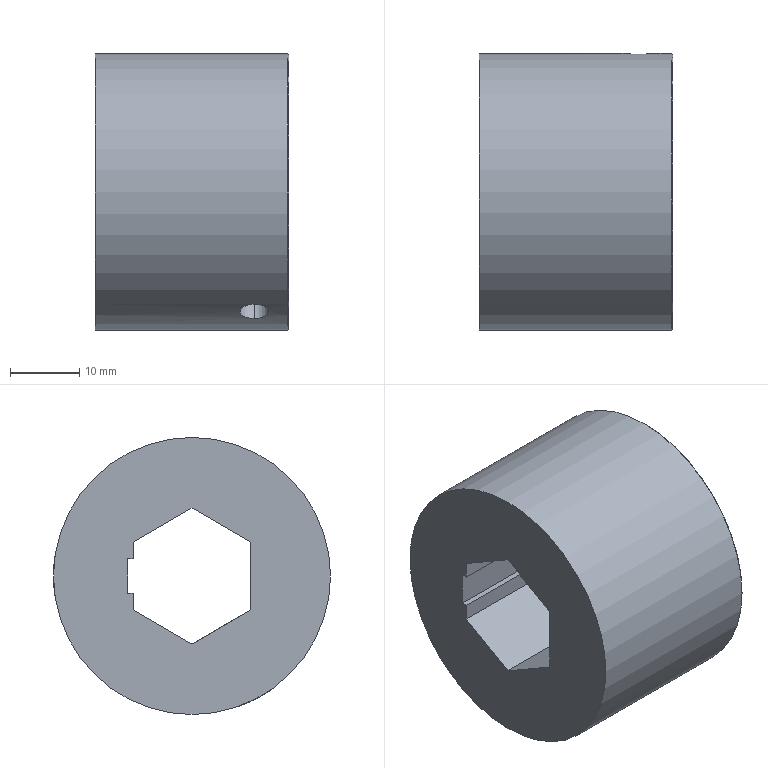Part | STEP file | ATP40XL050-B-hex socket | 1 solid | 19 faces | box 28 x 40 x 40 mm | volume 27766 mm3 | plane 12 | cylinder 5 | cone 2 | commonest cylinder face diameters 4.134 x4 40 x1
STEP:
#1=CARTESIAN_POINT('',(0.,8.5,-2.5));
#2=VERTEX_POINT('',#1);
#3=CARTESIAN_POINT('',(0.,8.5,-4.907));
#4=VERTEX_POINT('',#3);
#5=CARTESIAN_POINT('',(0.,8.5,0.));
#6=DIRECTION('',(0.,0.,-1.));
#7=VECTOR('',#6,1000.);
#8=LINE('',#5,#7);
#9=EDGE_CURVE('',#2,#4,#8,.T.);
#10=ORIENTED_EDGE('',*,*,#9,.F.);
#11=CARTESIAN_POINT('',(0.,9.3,-2.5));
#12=VERTEX_POINT('',#11);
#13=CARTESIAN_POINT('',(0.,13.65,-2.5));
#14=DIRECTION('',(0.,1.,0.));
#15=VECTOR('',#14,1000.);
#16=LINE('',#13,#15);
#17=EDGE_CURVE('',#2,#12,#16,.T.);
#18=ORIENTED_EDGE('',*,*,#17,.T.);
#19=CARTESIAN_POINT('',(0.,9.3,2.5));
#20=VERTEX_POINT('',#19);
#21=CARTESIAN_POINT('',(0.,9.3,1.25));
#22=DIRECTION('',(0.,0.,1.));
#23=VECTOR('',#22,1000.);
#24=LINE('',#21,#23);
#25=EDGE_CURVE('',#12,#20,#24,.T.);
#26=ORIENTED_EDGE('',*,*,#25,.T.);
#27=CARTESIAN_POINT('',(0.,8.5,2.5));
#28=VERTEX_POINT('',#27);
#29=CARTESIAN_POINT('',(0.,9.,2.5));
#30=DIRECTION('',(0.,-1.,0.));
#31=VECTOR('',#30,1000.);
#32=LINE('',#29,#31);
#33=EDGE_CURVE('',#20,#28,#32,.T.);
#34=ORIENTED_EDGE('',*,*,#33,.T.);
#35=CARTESIAN_POINT('',(0.,8.5,4.907));
#36=VERTEX_POINT('',#35);
#37=CARTESIAN_POINT('',(0.,8.5,4.907));
#38=DIRECTION('',(0.,0.,-1.));
#39=VECTOR('',#38,1000.);
#40=LINE('',#37,#39);
#41=EDGE_CURVE('',#36,#28,#40,.T.);
#42=ORIENTED_EDGE('',*,*,#41,.F.);
#43=CARTESIAN_POINT('',(0.,0.,9.815));
#44=VERTEX_POINT('',#43);
#45=CARTESIAN_POINT('',(0.,0.,9.815));
#46=DIRECTION('',(0.,0.866,-0.5));
#47=VECTOR('',#46,1000.);
#48=LINE('',#45,#47);
#49=EDGE_CURVE('',#44,#36,#48,.T.);
#50=ORIENTED_EDGE('',*,*,#49,.F.);
#51=CARTESIAN_POINT('',(0.,-8.5,4.907));
#52=VERTEX_POINT('',#51);
#53=CARTESIAN_POINT('',(0.,-8.5,4.907));
#54=DIRECTION('',(0.,0.866,0.5));
#55=VECTOR('',#54,1000.);
#56=LINE('',#53,#55);
#57=EDGE_CURVE('',#52,#44,#56,.T.);
#58=ORIENTED_EDGE('',*,*,#57,.F.);
#59=CARTESIAN_POINT('',(0.,-8.5,-4.907));
#60=VERTEX_POINT('',#59);
#61=CARTESIAN_POINT('',(0.,-8.5,-4.907));
#62=DIRECTION('',(0.,0.,1.));
#63=VECTOR('',#62,1000.);
#64=LINE('',#61,#63);
#65=EDGE_CURVE('',#60,#52,#64,.T.);
#66=ORIENTED_EDGE('',*,*,#65,.F.);
#67=CARTESIAN_POINT('',(0.,0.,-9.815));
#68=VERTEX_POINT('',#67);
#69=CARTESIAN_POINT('',(0.,0.,-9.815));
#70=DIRECTION('',(0.,-0.866,0.5));
#71=VECTOR('',#70,1000.);
#72=LINE('',#69,#71);
#73=EDGE_CURVE('',#68,#60,#72,.T.);
#74=ORIENTED_EDGE('',*,*,#73,.F.);
#75=CARTESIAN_POINT('',(0.,8.5,-4.907));
#76=DIRECTION('',(0.,-0.866,-0.5));
#77=VECTOR('',#76,1000.);
#78=LINE('',#75,#77);
#79=EDGE_CURVE('',#4,#68,#78,.T.);
#80=ORIENTED_EDGE('',*,*,#79,.F.);
#81=EDGE_LOOP('',(#10,#18,#26,#34,#42,#50,#58,#66,#74,#80));
#82=FACE_BOUND('',#81,.T.);
#83=CARTESIAN_POINT('',(0.,0.,-20.));
#84=VERTEX_POINT('',#83);
#85=CARTESIAN_POINT('',(0.,0.,0.));
#86=DIRECTION('',(1.,0.,0.));
#87=DIRECTION('',(0.,0.,-1.));
#88=AXIS2_PLACEMENT_3D('',#85,#86,#87);
#89=CIRCLE('',#88,20.);
#90=EDGE_CURVE('',#84,#84,#89,.T.);
#91=ORIENTED_EDGE('',*,*,#90,.F.);
#92=EDGE_LOOP('',(#91));
#93=FACE_OUTER_BOUND('',#92,.T.);
#94=CARTESIAN_POINT('',(0.,18.,0.));
#95=DIRECTION('',(-1.,0.,0.));
#96=DIRECTION('',(0.,0.,1.));
#97=AXIS2_PLACEMENT_3D('',#94,#95,#96);
#98=PLANE('',#97);
#99=ADVANCED_FACE('',(#82,#93),#98,.T.);
#100=CARTESIAN_POINT('',(28.,19.8,0.));
#101=VERTEX_POINT('',#100);
#102=CARTESIAN_POINT('',(27.8,20.,0.));
#103=VERTEX_POINT('',#102);
#104=CARTESIAN_POINT('',(27.9,19.9,0.));
#105=DIRECTION('',(-0.7071,0.7071,0.));
#106=VECTOR('',#105,1000.);
#107=LINE('',#104,#106);
#108=EDGE_CURVE('',#101,#103,#107,.T.);
#109=ORIENTED_EDGE('',*,*,#108,.F.);
#110=CARTESIAN_POINT('',(28.,-19.8,0.));
#111=VERTEX_POINT('',#110);
#112=CARTESIAN_POINT('',(28.,0.,0.));
#113=DIRECTION('',(-1.,0.,0.));
#114=DIRECTION('',(0.,1.,0.));
#115=AXIS2_PLACEMENT_3D('',#112,#113,#114);
#116=CIRCLE('',#115,19.8);
#117=EDGE_CURVE('',#101,#111,#116,.T.);
#118=ORIENTED_EDGE('',*,*,#117,.T.);
#119=CARTESIAN_POINT('',(27.8,-20.,0.));
#120=VERTEX_POINT('',#119);
#121=CARTESIAN_POINT('',(27.9,-19.9,0.));
#122=DIRECTION('',(0.7071,0.7071,0.));
#123=VECTOR('',#122,1000.);
#124=LINE('',#121,#123);
#125=EDGE_CURVE('',#120,#111,#124,.T.);
#126=ORIENTED_EDGE('',*,*,#125,.F.);
#127=CARTESIAN_POINT('',(27.8,0.,0.));
#128=DIRECTION('',(-1.,0.,0.));
#129=DIRECTION('',(0.,1.,0.));
#130=AXIS2_PLACEMENT_3D('',#127,#128,#129);
#131=CIRCLE('',#130,20.);
#132=EDGE_CURVE('',#103,#120,#131,.T.);
#133=ORIENTED_EDGE('',*,*,#132,.F.);
#134=EDGE_LOOP('',(#109,#118,#126,#133));
#135=FACE_OUTER_BOUND('',#134,.T.);
#136=CARTESIAN_POINT('',(27.9,0.,0.));
#137=DIRECTION('',(-1.,0.,0.));
#138=DIRECTION('',(0.,1.,0.));
#139=AXIS2_PLACEMENT_3D('',#136,#137,#138);
#140=CONICAL_SURFACE('',#139,19.9,0.7854);
#141=ADVANCED_FACE('',(#135),#140,.T.);
#142=CARTESIAN_POINT('',(23.,19.893,-2.067));
#143=VERTEX_POINT('',#142);
#144=CARTESIAN_POINT('',(25.067,20.,0.));
#145=VERTEX_POINT('',#144);
#146=CARTESIAN_POINT('',(23.,19.893,-2.067));
#147=CARTESIAN_POINT('',(23.274,19.893,-2.067));
#148=CARTESIAN_POINT('',(23.538,19.899,-2.014));
#149=CARTESIAN_POINT('',(24.044,19.919,-1.805));
#150=CARTESIAN_POINT('',(24.268,19.932,-1.655));
#151=CARTESIAN_POINT('',(24.655,19.961,-1.268));
#152=CARTESIAN_POINT('',(24.805,19.974,-1.045));
#153=CARTESIAN_POINT('',(25.015,19.994,-0.538));
#154=CARTESIAN_POINT('',(25.067,20.,-0.2742));
#155=CARTESIAN_POINT('',(25.067,20.,0.));
#156=B_SPLINE_CURVE_WITH_KNOTS('',3,(#146,#147,#148,#149,#150,#151,#152,#153,#154,#155),.UNSPECIFIED.,.F.,.F.,(4,2,2,2,4),(0.,0.25,0.5,0.75,1.),.UNSPECIFIED.);
#157=EDGE_CURVE('',#143,#145,#156,.T.);
#158=ORIENTED_EDGE('',*,*,#157,.T.);
#159=CARTESIAN_POINT('',(23.,19.893,2.067));
#160=VERTEX_POINT('',#159);
#161=CARTESIAN_POINT('',(25.067,20.,0.));
#162=CARTESIAN_POINT('',(25.067,20.,0.2741));
#163=CARTESIAN_POINT('',(25.014,19.994,0.5381));
#164=CARTESIAN_POINT('',(24.805,19.974,1.044));
#165=CARTESIAN_POINT('',(24.655,19.961,1.268));
#166=CARTESIAN_POINT('',(24.268,19.932,1.655));
#167=CARTESIAN_POINT('',(24.044,19.919,1.805));
#168=CARTESIAN_POINT('',(23.538,19.899,2.014));
#169=CARTESIAN_POINT('',(23.274,19.893,2.067));
#170=CARTESIAN_POINT('',(23.,19.893,2.067));
#171=B_SPLINE_CURVE_WITH_KNOTS('',3,(#161,#162,#163,#164,#165,#166,#167,#168,#169,#170),.UNSPECIFIED.,.F.,.F.,(4,2,2,2,4),(0.,0.25,0.5,0.75,1.),.UNSPECIFIED.);
#172=EDGE_CURVE('',#145,#160,#171,.T.);
#173=ORIENTED_EDGE('',*,*,#172,.T.);
#174=CARTESIAN_POINT('',(20.933,20.,0.));
#175=VERTEX_POINT('',#174);
#176=CARTESIAN_POINT('',(23.,19.893,2.067));
#177=CARTESIAN_POINT('',(22.726,19.893,2.067));
#178=CARTESIAN_POINT('',(22.462,19.899,2.014));
#179=CARTESIAN_POINT('',(21.956,19.919,1.805));
#180=CARTESIAN_POINT('',(21.732,19.932,1.655));
#181=CARTESIAN_POINT('',(21.345,19.961,1.268));
#182=CARTESIAN_POINT('',(21.195,19.974,1.045));
#183=CARTESIAN_POINT('',(20.985,19.994,0.538));
#184=CARTESIAN_POINT('',(20.933,20.,0.2742));
#185=CARTESIAN_POINT('',(20.933,20.,0.));
#186=B_SPLINE_CURVE_WITH_KNOTS('',3,(#176,#177,#178,#179,#180,#181,#182,#183,#184,#185),.UNSPECIFIED.,.F.,.F.,(4,2,2,2,4),(0.,0.25,0.5,0.75,1.),.UNSPECIFIED.);
#187=EDGE_CURVE('',#160,#175,#186,.T.);
#188=ORIENTED_EDGE('',*,*,#187,.T.);
#189=CARTESIAN_POINT('',(20.933,20.,0.));
#190=CARTESIAN_POINT('',(20.933,20.,-0.2741));
#191=CARTESIAN_POINT('',(20.986,19.994,-0.5381));
#192=CARTESIAN_POINT('',(21.195,19.974,-1.044));
#193=CARTESIAN_POINT('',(21.345,19.961,-1.268));
#194=CARTESIAN_POINT('',(21.732,19.932,-1.655));
#195=CARTESIAN_POINT('',(21.956,19.919,-1.805));
#196=CARTESIAN_POINT('',(22.462,19.899,-2.014));
#197=CARTESIAN_POINT('',(22.726,19.893,-2.067));
#198=CARTESIAN_POINT('',(23.,19.893,-2.067));
#199=B_SPLINE_CURVE_WITH_KNOTS('',3,(#189,#190,#191,#192,#193,#194,#195,#196,#197,#198),.UNSPECIFIED.,.F.,.F.,(4,2,2,2,4),(0.,0.25,0.5,0.75,1.),.UNSPECIFIED.);
#200=EDGE_CURVE('',#175,#143,#199,.T.);
#201=ORIENTED_EDGE('',*,*,#200,.T.);
#202=EDGE_LOOP('',(#158,#173,#188,#201));
#203=FACE_BOUND('',#202,.T.);
#204=ORIENTED_EDGE('',*,*,#132,.T.);
#205=CARTESIAN_POINT('',(27.8,0.,0.));
#206=DIRECTION('',(-1.,0.,0.));
#207=DIRECTION('',(0.,1.,0.));
#208=AXIS2_PLACEMENT_3D('',#205,#206,#207);
#209=CIRCLE('',#208,20.);
#210=EDGE_CURVE('',#120,#103,#209,.T.);
#211=ORIENTED_EDGE('',*,*,#210,.T.);
#212=EDGE_LOOP('',(#204,#211));
#213=FACE_OUTER_BOUND('',#212,.T.);
#214=CARTESIAN_POINT('',(25.067,-10.,-17.321));
#215=VERTEX_POINT('',#214);
#216=CARTESIAN_POINT('',(23.,-8.156,-18.261));
#217=VERTEX_POINT('',#216);
#218=CARTESIAN_POINT('',(25.067,-10.,-17.321));
#219=CARTESIAN_POINT('',(25.067,-9.763,-17.458));
#220=CARTESIAN_POINT('',(25.014,-9.531,-17.585));
#221=CARTESIAN_POINT('',(24.805,-9.083,-17.82));
#222=CARTESIAN_POINT('',(24.655,-8.882,-17.92));
#223=CARTESIAN_POINT('',(24.268,-8.533,-18.09));
#224=CARTESIAN_POINT('',(24.044,-8.397,-18.152));
#225=CARTESIAN_POINT('',(23.538,-8.205,-18.24));
#226=CARTESIAN_POINT('',(23.274,-8.156,-18.261));
#227=CARTESIAN_POINT('',(23.,-8.156,-18.261));
#228=B_SPLINE_CURVE_WITH_KNOTS('',3,(#218,#219,#220,#221,#222,#223,#224,#225,#226,#227),.UNSPECIFIED.,.F.,.F.,(4,2,2,2,4),(0.,0.25,0.5,0.75,1.),.UNSPECIFIED.);
#229=EDGE_CURVE('',#215,#217,#228,.T.);
#230=ORIENTED_EDGE('',*,*,#229,.T.);
#231=CARTESIAN_POINT('',(20.933,-10.,-17.321));
#232=VERTEX_POINT('',#231);
#233=CARTESIAN_POINT('',(23.,-8.156,-18.261));
#234=CARTESIAN_POINT('',(22.726,-8.156,-18.261));
#235=CARTESIAN_POINT('',(22.462,-8.205,-18.24));
#236=CARTESIAN_POINT('',(21.956,-8.396,-18.152));
#237=CARTESIAN_POINT('',(21.732,-8.533,-18.09));
#238=CARTESIAN_POINT('',(21.345,-8.882,-17.92));
#239=CARTESIAN_POINT('',(21.195,-9.083,-17.821));
#240=CARTESIAN_POINT('',(20.985,-9.531,-17.585));
#241=CARTESIAN_POINT('',(20.933,-9.763,-17.458));
#242=CARTESIAN_POINT('',(20.933,-10.,-17.321));
#243=B_SPLINE_CURVE_WITH_KNOTS('',3,(#233,#234,#235,#236,#237,#238,#239,#240,#241,#242),.UNSPECIFIED.,.F.,.F.,(4,2,2,2,4),(0.,0.25,0.5,0.75,1.),.UNSPECIFIED.);
#244=EDGE_CURVE('',#217,#232,#243,.T.);
#245=ORIENTED_EDGE('',*,*,#244,.T.);
#246=CARTESIAN_POINT('',(23.,-11.737,-16.194));
#247=VERTEX_POINT('',#246);
#248=CARTESIAN_POINT('',(20.933,-10.,-17.321));
#249=CARTESIAN_POINT('',(20.933,-10.237,-17.183));
#250=CARTESIAN_POINT('',(20.986,-10.463,-17.047));
#251=CARTESIAN_POINT('',(21.195,-10.892,-16.776));
#252=CARTESIAN_POINT('',(21.345,-11.078,-16.653));
#253=CARTESIAN_POINT('',(21.732,-11.4,-16.434));
#254=CARTESIAN_POINT('',(21.956,-11.522,-16.348));
#255=CARTESIAN_POINT('',(22.462,-11.694,-16.225));
#256=CARTESIAN_POINT('',(22.726,-11.736,-16.194));
#257=CARTESIAN_POINT('',(23.,-11.737,-16.194));
#258=B_SPLINE_CURVE_WITH_KNOTS('',3,(#248,#249,#250,#251,#252,#253,#254,#255,#256,#257),.UNSPECIFIED.,.F.,.F.,(4,2,2,2,4),(0.,0.25,0.5,0.75,1.),.UNSPECIFIED.);
#259=EDGE_CURVE('',#232,#247,#258,.T.);
#260=ORIENTED_EDGE('',*,*,#259,.T.);
#261=CARTESIAN_POINT('',(23.,-11.737,-16.194));
#262=CARTESIAN_POINT('',(23.274,-11.736,-16.194));
#263=CARTESIAN_POINT('',(23.538,-11.694,-16.225));
#264=CARTESIAN_POINT('',(24.044,-11.522,-16.348));
#265=CARTESIAN_POINT('',(24.268,-11.4,-16.434));
#266=CARTESIAN_POINT('',(24.655,-11.078,-16.653));
#267=CARTESIAN_POINT('',(24.805,-10.892,-16.776));
#268=CARTESIAN_POINT('',(25.015,-10.463,-17.047));
#269=CARTESIAN_POINT('',(25.067,-10.237,-17.183));
#270=CARTESIAN_POINT('',(25.067,-10.,-17.321));
#271=B_SPLINE_CURVE_WITH_KNOTS('',3,(#261,#262,#263,#264,#265,#266,#267,#268,#269,#270),.UNSPECIFIED.,.F.,.F.,(4,2,2,2,4),(0.,0.25,0.5,0.75,1.),.UNSPECIFIED.);
#272=EDGE_CURVE('',#247,#215,#271,.T.);
#273=ORIENTED_EDGE('',*,*,#272,.T.);
#274=EDGE_LOOP('',(#230,#245,#260,#273));
#275=FACE_BOUND('',#274,.T.);
#276=ORIENTED_EDGE('',*,*,#90,.T.);
#277=EDGE_LOOP('',(#276));
#278=FACE_OUTER_BOUND('',#277,.T.);
#279=CARTESIAN_POINT('',(23.4,0.,0.));
#280=DIRECTION('',(1.,0.,0.));
#281=DIRECTION('',(0.,1.,0.));
#282=AXIS2_PLACEMENT_3D('',#279,#280,#281);
#283=CYLINDRICAL_SURFACE('',#282,20.);
#284=ADVANCED_FACE('',(#203,#213,#275,#278),#283,.T.);
#285=CARTESIAN_POINT('',(23.,9.3,2.067));
#286=VERTEX_POINT('',#285);
#287=CARTESIAN_POINT('',(23.,14.65,2.067));
#288=DIRECTION('',(0.,1.,0.));
#289=VECTOR('',#288,1000.);
#290=LINE('',#287,#289);
#291=EDGE_CURVE('',#286,#160,#290,.T.);
#292=ORIENTED_EDGE('',*,*,#291,.F.);
#293=CARTESIAN_POINT('',(23.,9.3,-2.067));
#294=VERTEX_POINT('',#293);
#295=CARTESIAN_POINT('',(23.,9.3,0.));
#296=DIRECTION('',(0.,1.,0.));
#297=DIRECTION('',(0.,0.,1.));
#298=AXIS2_PLACEMENT_3D('',#295,#296,#297);
#299=CIRCLE('',#298,2.067);
#300=EDGE_CURVE('',#294,#286,#299,.T.);
#301=ORIENTED_EDGE('',*,*,#300,.F.);
#302=CARTESIAN_POINT('',(23.,14.65,-2.067));
#303=DIRECTION('',(0.,-1.,0.));
#304=VECTOR('',#303,1000.);
#305=LINE('',#302,#304);
#306=EDGE_CURVE('',#143,#294,#305,.T.);
#307=ORIENTED_EDGE('',*,*,#306,.F.);
#308=ORIENTED_EDGE('',*,*,#200,.F.);
#309=ORIENTED_EDGE('',*,*,#187,.F.);
#310=EDGE_LOOP('',(#292,#301,#307,#308,#309));
#311=FACE_OUTER_BOUND('',#310,.T.);
#312=CARTESIAN_POINT('',(23.,14.65,0.));
#313=DIRECTION('',(0.,1.,0.));
#314=DIRECTION('',(0.,0.,1.));
#315=AXIS2_PLACEMENT_3D('',#312,#313,#314);
#316=CYLINDRICAL_SURFACE('',#315,2.067);
#317=ADVANCED_FACE('',(#311),#316,.F.);
#318=CARTESIAN_POINT('',(23.,-2.46,-8.395));
#319=VERTEX_POINT('',#318);
#320=CARTESIAN_POINT('',(23.,-4.71,-12.292));
#321=DIRECTION('',(0.,-0.5,-0.866));
#322=VECTOR('',#321,1000.);
#323=LINE('',#320,#322);
#324=EDGE_CURVE('',#319,#217,#323,.T.);
#325=ORIENTED_EDGE('',*,*,#324,.F.);
#326=CARTESIAN_POINT('',(23.,-6.04,-6.328));
#327=VERTEX_POINT('',#326);
#328=CARTESIAN_POINT('',(23.,-4.25,-7.361));
#329=DIRECTION('',(0.,0.5,0.866));
#330=DIRECTION('',(0.,0.866,-0.5));
#331=AXIS2_PLACEMENT_3D('',#328,#329,#330);
#332=CIRCLE('',#331,2.067);
#333=EDGE_CURVE('',#319,#327,#332,.T.);
#334=ORIENTED_EDGE('',*,*,#333,.T.);
#335=CARTESIAN_POINT('',(23.,-8.29,-10.225));
#336=DIRECTION('',(0.,0.5,0.866));
#337=VECTOR('',#336,1000.);
#338=LINE('',#335,#337);
#339=EDGE_CURVE('',#247,#327,#338,.T.);
#340=ORIENTED_EDGE('',*,*,#339,.F.);
#341=ORIENTED_EDGE('',*,*,#259,.F.);
#342=ORIENTED_EDGE('',*,*,#244,.F.);
#343=EDGE_LOOP('',(#325,#334,#340,#341,#342));
#344=FACE_OUTER_BOUND('',#343,.T.);
#345=CARTESIAN_POINT('',(23.,-6.5,-11.258));
#346=DIRECTION('',(0.,0.5,0.866));
#347=DIRECTION('',(0.,-0.866,0.5));
#348=AXIS2_PLACEMENT_3D('',#345,#346,#347);
#349=CYLINDRICAL_SURFACE('',#348,2.067);
#350=ADVANCED_FACE('',(#344),#349,.F.);
#351=ORIENTED_EDGE('',*,*,#339,.T.);
#352=CARTESIAN_POINT('',(23.,-4.25,-7.361));
#353=DIRECTION('',(0.,0.5,0.866));
#354=DIRECTION('',(0.,0.866,-0.5));
#355=AXIS2_PLACEMENT_3D('',#352,#353,#354);
#356=CIRCLE('',#355,2.067);
#357=EDGE_CURVE('',#327,#319,#356,.T.);
#358=ORIENTED_EDGE('',*,*,#357,.T.);
#359=ORIENTED_EDGE('',*,*,#324,.T.);
#360=ORIENTED_EDGE('',*,*,#229,.F.);
#361=ORIENTED_EDGE('',*,*,#272,.F.);
#362=EDGE_LOOP('',(#351,#358,#359,#360,#361));
#363=FACE_OUTER_BOUND('',#362,.T.);
#364=CARTESIAN_POINT('',(23.,-6.5,-11.258));
#365=DIRECTION('',(0.,0.5,0.866));
#366=DIRECTION('',(0.,-0.866,0.5));
#367=AXIS2_PLACEMENT_3D('',#364,#365,#366);
#368=CYLINDRICAL_SURFACE('',#367,2.067);
#369=ADVANCED_FACE('',(#363),#368,.F.);
#370=ORIENTED_EDGE('',*,*,#291,.T.);
#371=ORIENTED_EDGE('',*,*,#172,.F.);
#372=ORIENTED_EDGE('',*,*,#157,.F.);
#373=ORIENTED_EDGE('',*,*,#306,.T.);
#374=CARTESIAN_POINT('',(23.,9.3,0.));
#375=DIRECTION('',(0.,1.,0.));
#376=DIRECTION('',(0.,0.,1.));
#377=AXIS2_PLACEMENT_3D('',#374,#375,#376);
#378=CIRCLE('',#377,2.067);
#379=EDGE_CURVE('',#286,#294,#378,.T.);
#380=ORIENTED_EDGE('',*,*,#379,.F.);
#381=EDGE_LOOP('',(#370,#371,#372,#373,#380));
#382=FACE_OUTER_BOUND('',#381,.T.);
#383=CARTESIAN_POINT('',(23.,14.65,0.));
#384=DIRECTION('',(0.,1.,0.));
#385=DIRECTION('',(0.,0.,1.));
#386=AXIS2_PLACEMENT_3D('',#383,#384,#385);
#387=CYLINDRICAL_SURFACE('',#386,2.067);
#388=ADVANCED_FACE('',(#382),#387,.F.);
#389=ORIENTED_EDGE('',*,*,#17,.F.);
#390=CARTESIAN_POINT('',(28.,8.5,-2.5));
#391=VERTEX_POINT('',#390);
#392=CARTESIAN_POINT('',(0.,8.5,-2.5));
#393=DIRECTION('',(1.,0.,0.));
#394=VECTOR('',#393,1000.);
#395=LINE('',#392,#394);
#396=EDGE_CURVE('',#2,#391,#395,.T.);
#397=ORIENTED_EDGE('',*,*,#396,.T.);
#398=CARTESIAN_POINT('',(28.,9.3,-2.5));
#399=VERTEX_POINT('',#398);
#400=CARTESIAN_POINT('',(28.,11.4,-2.5));
#401=DIRECTION('',(0.,-1.,0.));
#402=VECTOR('',#401,1000.);
#403=LINE('',#400,#402);
#404=EDGE_CURVE('',#399,#391,#403,.T.);
#405=ORIENTED_EDGE('',*,*,#404,.F.);
#406=CARTESIAN_POINT('',(0.,9.3,-2.5));
#407=DIRECTION('',(1.,0.,0.));
#408=VECTOR('',#407,1000.);
#409=LINE('',#406,#408);
#410=EDGE_CURVE('',#12,#399,#409,.T.);
#411=ORIENTED_EDGE('',*,*,#410,.F.);
#412=EDGE_LOOP('',(#389,#397,#405,#411));
#413=FACE_OUTER_BOUND('',#412,.T.);
#414=CARTESIAN_POINT('',(0.,9.3,-2.5));
#415=DIRECTION('',(0.,0.,-1.));
#416=DIRECTION('',(0.,-1.,0.));
#417=AXIS2_PLACEMENT_3D('',#414,#415,#416);
#418=PLANE('',#417);
#419=ADVANCED_FACE('',(#413),#418,.F.);
#420=CARTESIAN_POINT('',(28.,8.5,2.5));
#421=VERTEX_POINT('',#420);
#422=CARTESIAN_POINT('',(28.,9.3,2.5));
#423=VERTEX_POINT('',#422);
#424=CARTESIAN_POINT('',(28.,6.75,2.5));
#425=DIRECTION('',(0.,1.,0.));
#426=VECTOR('',#425,1000.);
#427=LINE('',#424,#426);
#428=EDGE_CURVE('',#421,#423,#427,.T.);
#429=ORIENTED_EDGE('',*,*,#428,.F.);
#430=CARTESIAN_POINT('',(0.,8.5,2.5));
#431=DIRECTION('',(-1.,0.,0.));
#432=VECTOR('',#431,1000.);
#433=LINE('',#430,#432);
#434=EDGE_CURVE('',#421,#28,#433,.T.);
#435=ORIENTED_EDGE('',*,*,#434,.T.);
#436=ORIENTED_EDGE('',*,*,#33,.F.);
#437=CARTESIAN_POINT('',(0.,9.3,2.5));
#438=DIRECTION('',(1.,0.,0.));
#439=VECTOR('',#438,1000.);
#440=LINE('',#437,#439);
#441=EDGE_CURVE('',#20,#423,#440,.T.);
#442=ORIENTED_EDGE('',*,*,#441,.T.);
#443=EDGE_LOOP('',(#429,#435,#436,#442));
#444=FACE_OUTER_BOUND('',#443,.T.);
#445=CARTESIAN_POINT('',(0.,0.,2.5));
#446=DIRECTION('',(0.,0.,1.));
#447=DIRECTION('',(1.,0.,0.));
#448=AXIS2_PLACEMENT_3D('',#445,#446,#447);
#449=PLANE('',#448);
#450=ADVANCED_FACE('',(#444),#449,.F.);
#451=CARTESIAN_POINT('',(28.,9.3,1.25));
#452=DIRECTION('',(0.,0.,-1.));
#453=VECTOR('',#452,1000.);
#454=LINE('',#451,#453);
#455=EDGE_CURVE('',#423,#399,#454,.T.);
#456=ORIENTED_EDGE('',*,*,#455,.F.);
#457=ORIENTED_EDGE('',*,*,#441,.F.);
#458=ORIENTED_EDGE('',*,*,#25,.F.);
#459=ORIENTED_EDGE('',*,*,#410,.T.);
#460=EDGE_LOOP('',(#456,#457,#458,#459));
#461=FACE_OUTER_BOUND('',#460,.T.);
#462=ORIENTED_EDGE('',*,*,#379,.T.);
#463=ORIENTED_EDGE('',*,*,#300,.T.);
#464=EDGE_LOOP('',(#462,#463));
#465=FACE_BOUND('',#464,.T.);
#466=CARTESIAN_POINT('',(0.,9.3,2.5));
#467=DIRECTION('',(0.,1.,0.));
#468=DIRECTION('',(1.,0.,0.));
#469=AXIS2_PLACEMENT_3D('',#466,#467,#468);
#470=PLANE('',#469);
#471=ADVANCED_FACE('',(#461,#465),#470,.F.);
#472=CARTESIAN_POINT('',(28.,8.5,-4.907));
#473=VERTEX_POINT('',#472);
#474=CARTESIAN_POINT('',(28.,8.5,4.907));
#475=DIRECTION('',(0.,0.,-1.));
#476=VECTOR('',#475,1000.);
#477=LINE('',#474,#476);
#478=EDGE_CURVE('',#391,#473,#477,.T.);
#479=ORIENTED_EDGE('',*,*,#478,.T.);
#480=CARTESIAN_POINT('',(28.,0.,-9.815));
#481=VERTEX_POINT('',#480);
#482=CARTESIAN_POINT('',(28.,8.5,-4.907));
#483=DIRECTION('',(0.,-0.866,-0.5));
#484=VECTOR('',#483,1000.);
#485=LINE('',#482,#484);
#486=EDGE_CURVE('',#473,#481,#485,.T.);
#487=ORIENTED_EDGE('',*,*,#486,.T.);
#488=CARTESIAN_POINT('',(28.,-8.5,-4.907));
#489=VERTEX_POINT('',#488);
#490=CARTESIAN_POINT('',(28.,0.,-9.815));
#491=DIRECTION('',(0.,-0.866,0.5));
#492=VECTOR('',#491,1000.);
#493=LINE('',#490,#492);
#494=EDGE_CURVE('',#481,#489,#493,.T.);
#495=ORIENTED_EDGE('',*,*,#494,.T.);
#496=CARTESIAN_POINT('',(28.,-8.5,4.907));
#497=VERTEX_POINT('',#496);
#498=CARTESIAN_POINT('',(28.,-8.5,-4.907));
#499=DIRECTION('',(0.,0.,1.));
#500=VECTOR('',#499,1000.);
#501=LINE('',#498,#500);
#502=EDGE_CURVE('',#489,#497,#501,.T.);
#503=ORIENTED_EDGE('',*,*,#502,.T.);
#504=CARTESIAN_POINT('',(28.,0.,9.815));
#505=VERTEX_POINT('',#504);
#506=CARTESIAN_POINT('',(28.,-8.5,4.907));
#507=DIRECTION('',(0.,0.866,0.5));
#508=VECTOR('',#507,1000.);
#509=LINE('',#506,#508);
#510=EDGE_CURVE('',#497,#505,#509,.T.);
#511=ORIENTED_EDGE('',*,*,#510,.T.);
#512=CARTESIAN_POINT('',(28.,8.5,4.907));
#513=VERTEX_POINT('',#512);
#514=CARTESIAN_POINT('',(28.,0.,9.815));
#515=DIRECTION('',(0.,0.866,-0.5));
#516=VECTOR('',#515,1000.);
#517=LINE('',#514,#516);
#518=EDGE_CURVE('',#505,#513,#517,.T.);
#519=ORIENTED_EDGE('',*,*,#518,.T.);
#520=CARTESIAN_POINT('',(28.,8.5,4.907));
#521=DIRECTION('',(0.,0.,-1.));
#522=VECTOR('',#521,1000.);
#523=LINE('',#520,#522);
#524=EDGE_CURVE('',#513,#421,#523,.T.);
#525=ORIENTED_EDGE('',*,*,#524,.T.);
#526=ORIENTED_EDGE('',*,*,#428,.T.);
#527=ORIENTED_EDGE('',*,*,#455,.T.);
#528=ORIENTED_EDGE('',*,*,#404,.T.);
#529=EDGE_LOOP('',(#479,#487,#495,#503,#511,#519,#525,#526,#527,#528));
#530=FACE_BOUND('',#529,.T.);
#531=ORIENTED_EDGE('',*,*,#117,.F.);
#532=CARTESIAN_POINT('',(28.,0.,0.));
#533=DIRECTION('',(-1.,0.,0.));
#534=DIRECTION('',(0.,1.,0.));
#535=AXIS2_PLACEMENT_3D('',#532,#533,#534);
#536=CIRCLE('',#535,19.8);
#537=EDGE_CURVE('',#111,#101,#536,.T.);
#538=ORIENTED_EDGE('',*,*,#537,.F.);
#539=EDGE_LOOP('',(#531,#538));
#540=FACE_OUTER_BOUND('',#539,.T.);
#541=CARTESIAN_POINT('',(28.,13.5,0.));
#542=DIRECTION('',(1.,0.,0.));
#543=DIRECTION('',(0.,1.,0.));
#544=AXIS2_PLACEMENT_3D('',#541,#542,#543);
#545=PLANE('',#544);
#546=ADVANCED_FACE('',(#530,#540),#545,.T.);
#547=ORIENTED_EDGE('',*,*,#108,.T.);
#548=ORIENTED_EDGE('',*,*,#210,.F.);
#549=ORIENTED_EDGE('',*,*,#125,.T.);
#550=ORIENTED_EDGE('',*,*,#537,.T.);
#551=EDGE_LOOP('',(#547,#548,#549,#550));
#552=FACE_OUTER_BOUND('',#551,.T.);
#553=CARTESIAN_POINT('',(27.9,0.,0.));
#554=DIRECTION('',(-1.,0.,0.));
#555=DIRECTION('',(0.,1.,0.));
#556=AXIS2_PLACEMENT_3D('',#553,#554,#555);
#557=CONICAL_SURFACE('',#556,19.9,0.7854);
#558=ADVANCED_FACE('',(#552),#557,.T.);
#559=ORIENTED_EDGE('',*,*,#73,.T.);
#560=CARTESIAN_POINT('',(28.,-8.5,-4.907));
#561=DIRECTION('',(-1.,0.,0.));
#562=VECTOR('',#561,1000.);
#563=LINE('',#560,#562);
#564=EDGE_CURVE('',#489,#60,#563,.T.);
#565=ORIENTED_EDGE('',*,*,#564,.F.);
#566=ORIENTED_EDGE('',*,*,#494,.F.);
#567=CARTESIAN_POINT('',(28.,0.,-9.815));
#568=DIRECTION('',(-1.,0.,0.));
#569=VECTOR('',#568,1000.);
#570=LINE('',#567,#569);
#571=EDGE_CURVE('',#481,#68,#570,.T.);
#572=ORIENTED_EDGE('',*,*,#571,.T.);
#573=EDGE_LOOP('',(#559,#565,#566,#572));
#574=FACE_OUTER_BOUND('',#573,.T.);
#575=ORIENTED_EDGE('',*,*,#357,.F.);
#576=ORIENTED_EDGE('',*,*,#333,.F.);
#577=EDGE_LOOP('',(#575,#576));
#578=FACE_BOUND('',#577,.T.);
#579=CARTESIAN_POINT('',(28.,0.,-9.815));
#580=DIRECTION('',(0.,-0.5,-0.866));
#581=DIRECTION('',(0.,0.866,-0.5));
#582=AXIS2_PLACEMENT_3D('',#579,#580,#581);
#583=PLANE('',#582);
#584=ADVANCED_FACE('',(#574,#578),#583,.F.);
#585=ORIENTED_EDGE('',*,*,#9,.T.);
#586=CARTESIAN_POINT('',(28.,8.5,-4.907));
#587=DIRECTION('',(-1.,0.,0.));
#588=VECTOR('',#587,1000.);
#589=LINE('',#586,#588);
#590=EDGE_CURVE('',#473,#4,#589,.T.);
#591=ORIENTED_EDGE('',*,*,#590,.F.);
#592=ORIENTED_EDGE('',*,*,#478,.F.);
#593=ORIENTED_EDGE('',*,*,#396,.F.);
#594=EDGE_LOOP('',(#585,#591,#592,#593));
#595=FACE_OUTER_BOUND('',#594,.T.);
#596=CARTESIAN_POINT('',(28.,8.5,4.907));
#597=DIRECTION('',(0.,1.,0.));
#598=DIRECTION('',(0.,0.,1.));
#599=AXIS2_PLACEMENT_3D('',#596,#597,#598);
#600=PLANE('',#599);
#601=ADVANCED_FACE('',(#595),#600,.F.);
#602=ORIENTED_EDGE('',*,*,#524,.F.);
#603=CARTESIAN_POINT('',(28.,8.5,4.907));
#604=DIRECTION('',(-1.,0.,0.));
#605=VECTOR('',#604,1000.);
#606=LINE('',#603,#605);
#607=EDGE_CURVE('',#513,#36,#606,.T.);
#608=ORIENTED_EDGE('',*,*,#607,.T.);
#609=ORIENTED_EDGE('',*,*,#41,.T.);
#610=ORIENTED_EDGE('',*,*,#434,.F.);
#611=EDGE_LOOP('',(#602,#608,#609,#610));
#612=FACE_OUTER_BOUND('',#611,.T.);
#613=CARTESIAN_POINT('',(28.,8.5,4.907));
#614=DIRECTION('',(0.,1.,0.));
#615=DIRECTION('',(0.,0.,1.));
#616=AXIS2_PLACEMENT_3D('',#613,#614,#615);
#617=PLANE('',#616);
#618=ADVANCED_FACE('',(#612),#617,.F.);
#619=ORIENTED_EDGE('',*,*,#57,.T.);
#620=CARTESIAN_POINT('',(28.,0.,9.815));
#621=DIRECTION('',(-1.,0.,0.));
#622=VECTOR('',#621,1000.);
#623=LINE('',#620,#622);
#624=EDGE_CURVE('',#505,#44,#623,.T.);
#625=ORIENTED_EDGE('',*,*,#624,.F.);
#626=ORIENTED_EDGE('',*,*,#510,.F.);
#627=CARTESIAN_POINT('',(28.,-8.5,4.907));
#628=DIRECTION('',(-1.,0.,0.));
#629=VECTOR('',#628,1000.);
#630=LINE('',#627,#629);
#631=EDGE_CURVE('',#497,#52,#630,.T.);
#632=ORIENTED_EDGE('',*,*,#631,.T.);
#633=EDGE_LOOP('',(#619,#625,#626,#632));
#634=FACE_OUTER_BOUND('',#633,.T.);
#635=CARTESIAN_POINT('',(28.,-8.5,4.907));
#636=DIRECTION('',(0.,-0.5,0.866));
#637=DIRECTION('',(0.,-0.866,-0.5));
#638=AXIS2_PLACEMENT_3D('',#635,#636,#637);
#639=PLANE('',#638);
#640=ADVANCED_FACE('',(#634),#639,.F.);
#641=ORIENTED_EDGE('',*,*,#65,.T.);
#642=ORIENTED_EDGE('',*,*,#631,.F.);
#643=ORIENTED_EDGE('',*,*,#502,.F.);
#644=ORIENTED_EDGE('',*,*,#564,.T.);
#645=EDGE_LOOP('',(#641,#642,#643,#644));
#646=FACE_OUTER_BOUND('',#645,.T.);
#647=CARTESIAN_POINT('',(28.,-8.5,-4.907));
#648=DIRECTION('',(0.,-1.,0.));
#649=DIRECTION('',(0.,0.,-1.));
#650=AXIS2_PLACEMENT_3D('',#647,#648,#649);
#651=PLANE('',#650);
#652=ADVANCED_FACE('',(#646),#651,.F.);
#653=ORIENTED_EDGE('',*,*,#79,.T.);
#654=ORIENTED_EDGE('',*,*,#571,.F.);
#655=ORIENTED_EDGE('',*,*,#486,.F.);
#656=ORIENTED_EDGE('',*,*,#590,.T.);
#657=EDGE_LOOP('',(#653,#654,#655,#656));
#658=FACE_OUTER_BOUND('',#657,.T.);
#659=CARTESIAN_POINT('',(28.,8.5,-4.907));
#660=DIRECTION('',(0.,0.5,-0.866));
#661=DIRECTION('',(0.,0.866,0.5));
#662=AXIS2_PLACEMENT_3D('',#659,#660,#661);
#663=PLANE('',#662);
#664=ADVANCED_FACE('',(#658),#663,.F.);
#665=ORIENTED_EDGE('',*,*,#49,.T.);
#666=ORIENTED_EDGE('',*,*,#607,.F.);
#667=ORIENTED_EDGE('',*,*,#518,.F.);
#668=ORIENTED_EDGE('',*,*,#624,.T.);
#669=EDGE_LOOP('',(#665,#666,#667,#668));
#670=FACE_OUTER_BOUND('',#669,.T.);
#671=CARTESIAN_POINT('',(28.,0.,9.815));
#672=DIRECTION('',(0.,0.5,0.866));
#673=DIRECTION('',(0.,-0.866,0.5));
#674=AXIS2_PLACEMENT_3D('',#671,#672,#673);
#675=PLANE('',#674);
#676=ADVANCED_FACE('',(#670),#675,.F.);
#677=CLOSED_SHELL('',(#99,#141,#284,#317,#350,#369,#388,#419,#450,#471,#546,#558,#584,#601,#618,#640,#652,#664,#676));
#678=MANIFOLD_SOLID_BREP('',#677);
#679=CARTESIAN_POINT('',(0.,0.,0.));
#680=DIRECTION('',(0.,0.,1.));
#681=DIRECTION('',(1.,0.,0.));
#682=AXIS2_PLACEMENT_3D('',#679,#680,#681);
#683=(LENGTH_UNIT()NAMED_UNIT(*)SI_UNIT(.MILLI.,.METRE.));
#684=UNCERTAINTY_MEASURE_WITH_UNIT(LENGTH_MEASURE(0.00001),#683,'','');
#685=(NAMED_UNIT(*)PLANE_ANGLE_UNIT()SI_UNIT($,.RADIAN.));
#686=(NAMED_UNIT(*)SI_UNIT($,.STERADIAN.)SOLID_ANGLE_UNIT());
#687=(GEOMETRIC_REPRESENTATION_CONTEXT(3)GLOBAL_UNCERTAINTY_ASSIGNED_CONTEXT((#684))GLOBAL_UNIT_ASSIGNED_CONTEXT((#683,#685,#686))REPRESENTATION_CONTEXT('',''));
#688=ADVANCED_BREP_SHAPE_REPRESENTATION('',(#678,#682),#687);